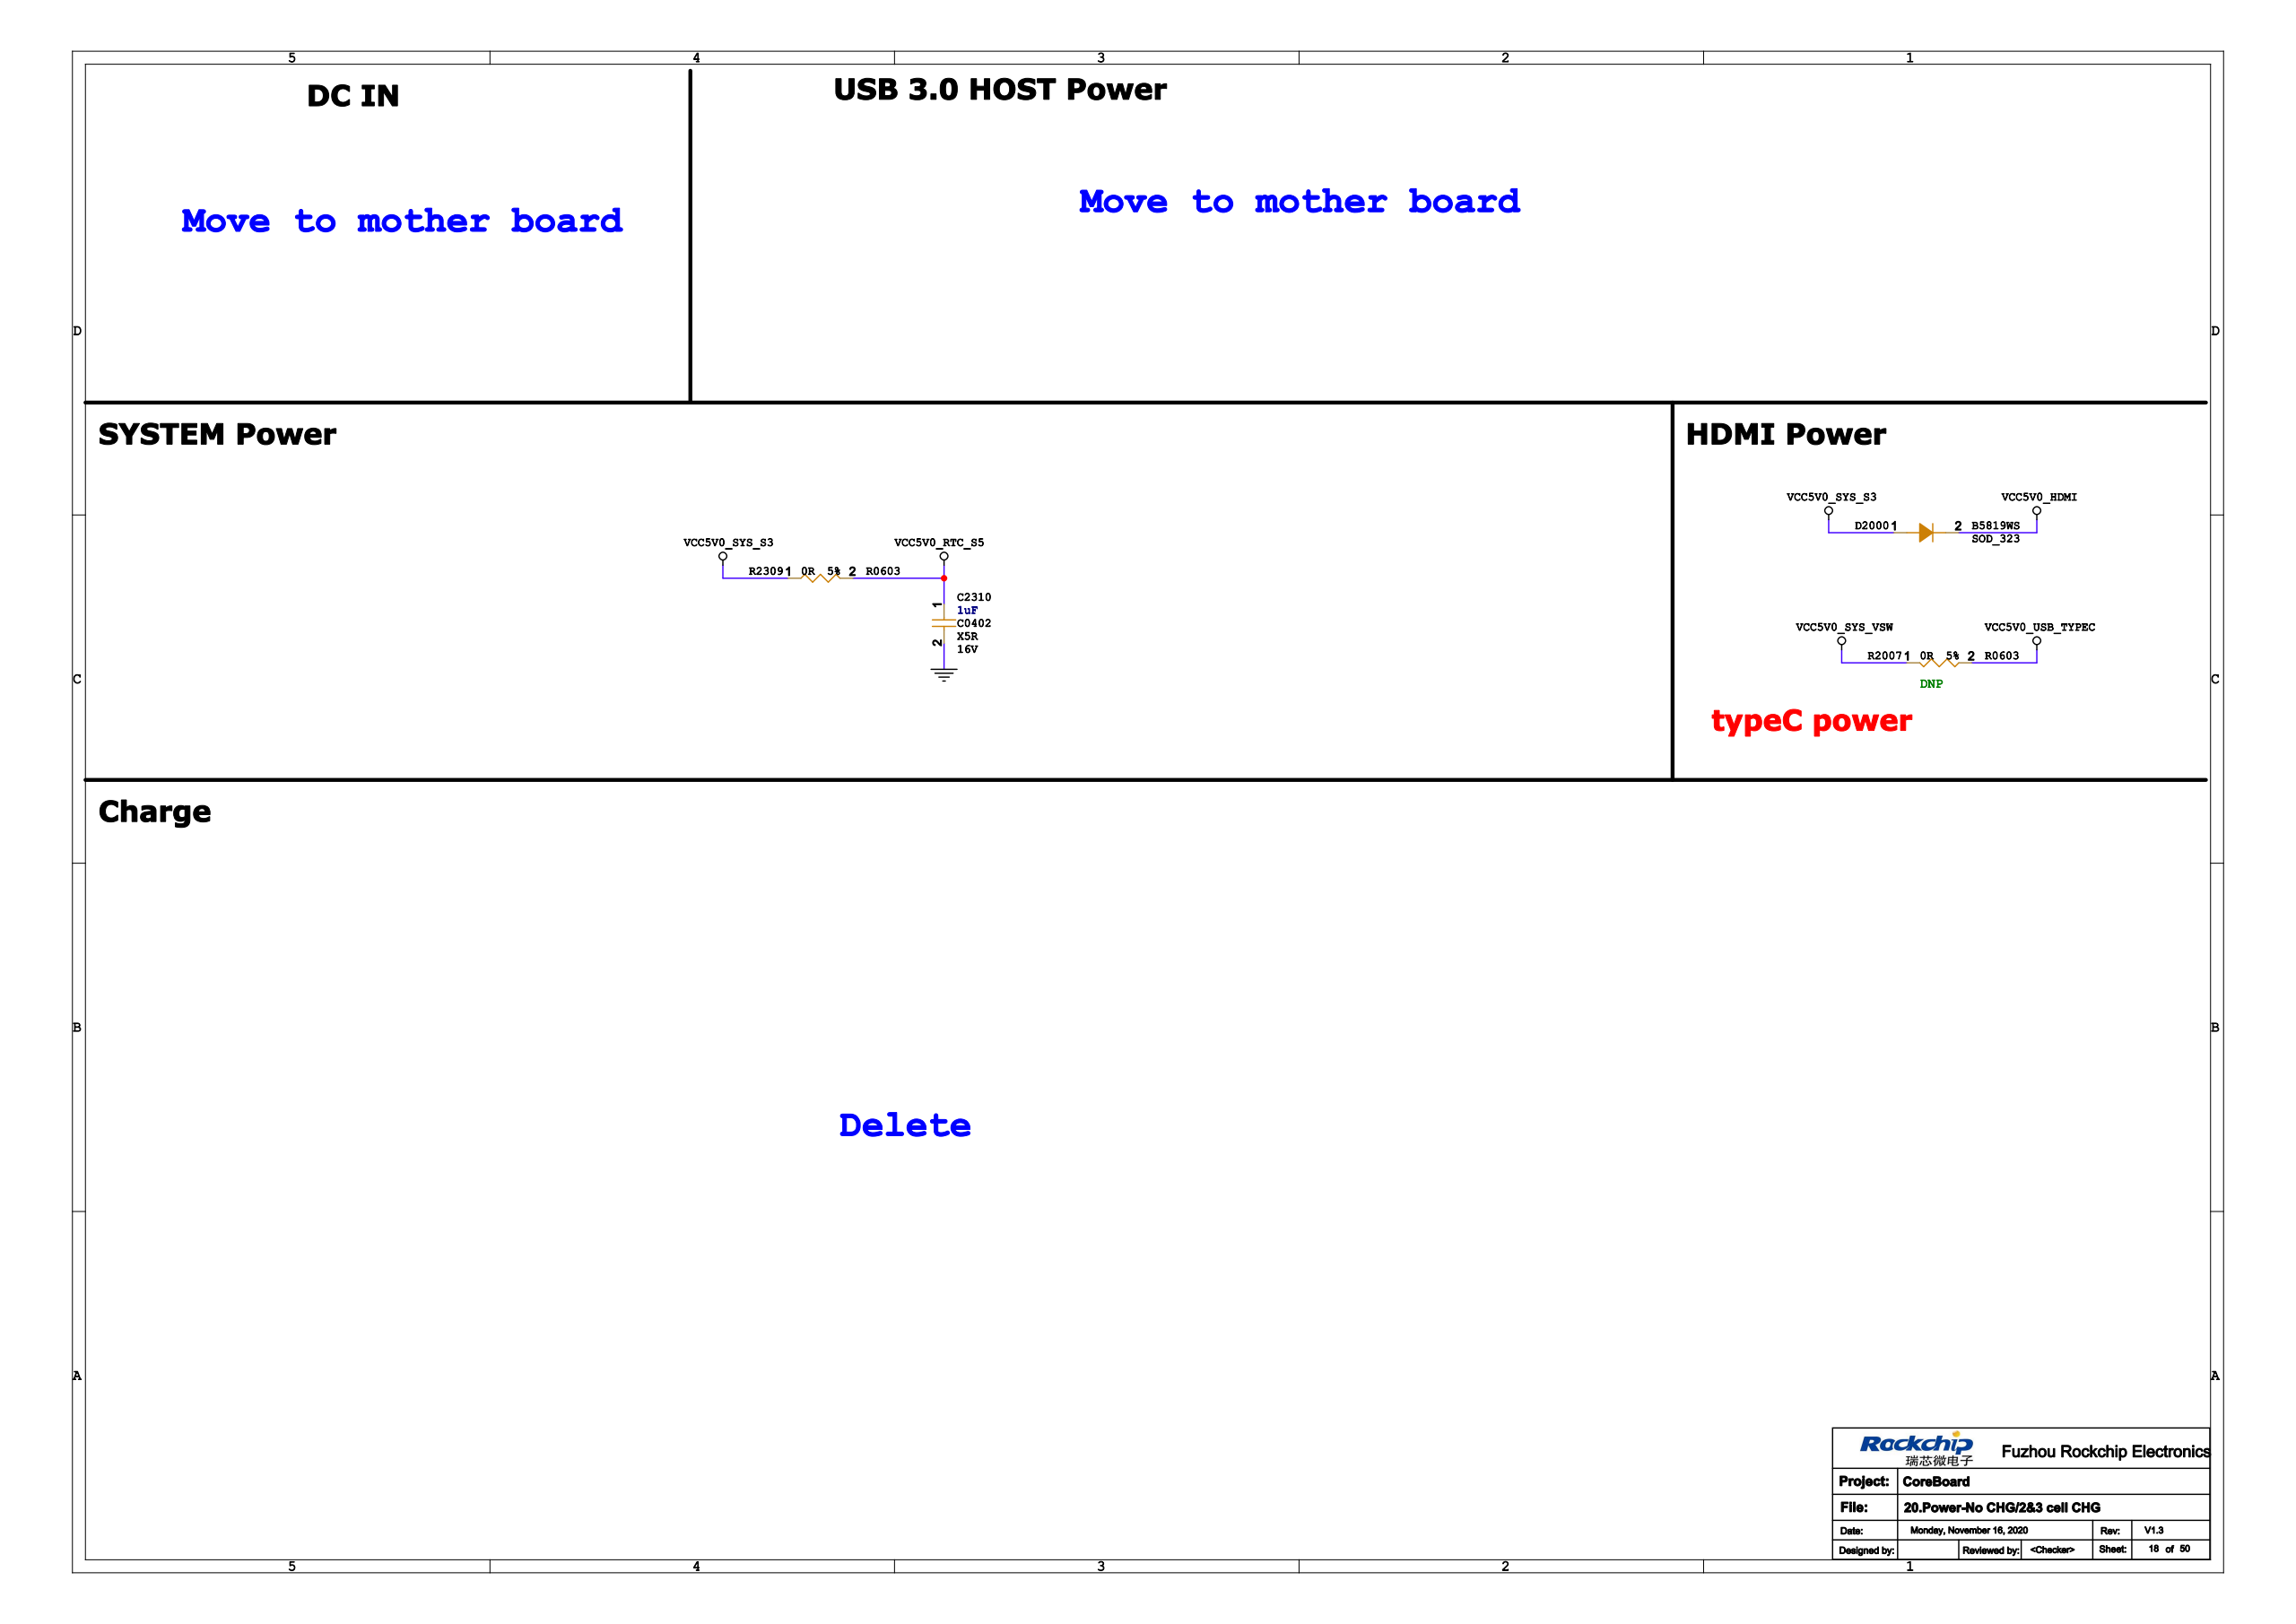Circuit board | Cadence Allegro | 749 parts | 717 nets | one sheet of the schematic
Parts on this sheet (reference | value | footprint):
C2310 | 1uF | C0402
D2000 | B5819WS | SOD_323
R2007 | 0R | R0603
Nets of these parts (net: part-pin ...):
GND: C2310-2
VCC5V0_USB_TYPEC: R2007-2
VCC5V0_SYS_VSW: R2007-1
VCC5V0_SYS_S3: D2000-1
VCC5V0_HDMI: D2000-2
VCC5V0_RTC_S5: C2310-1